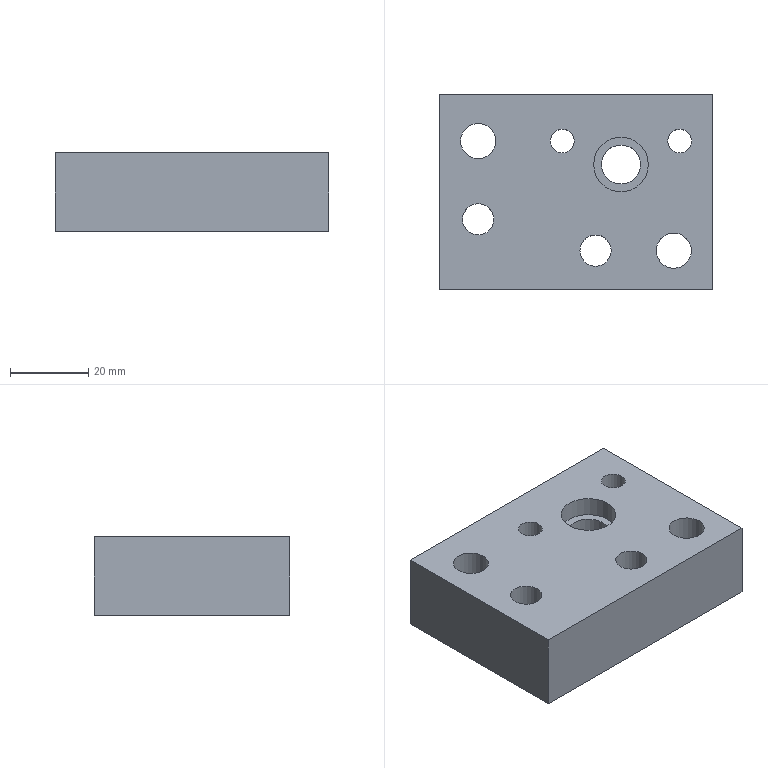Part | STEP file | 424_id2490_x_t | 1 solid | 23 faces | box 70 x 50 x 20 mm | volume 59956 mm3 | cylinder 12 | plane 11 | commonest cylinder face diameters 10 x3 14 x3 6.1 x2 8 x2 9 x2